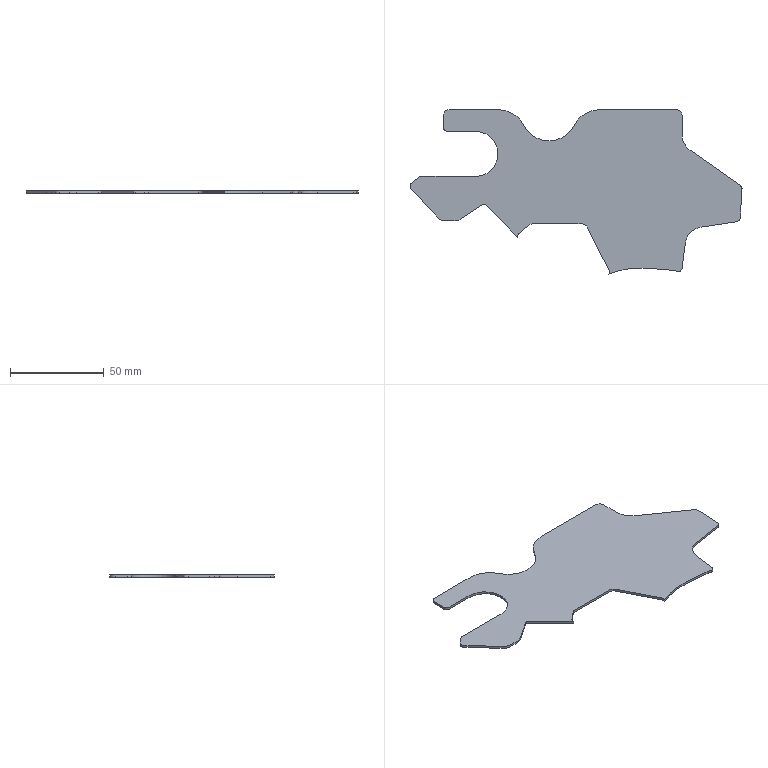Part | STEP file | gslz 2016.10.28-13_id246_x_t | 1 solid | 47 faces | box 176.605 x 87.506 x 1.25 mm | volume 11147 mm3 | cylinder 24 | plane 23 | commonest cylinder face diameters 4 x9 6 x5 30 x4 20 x2 3 x1 12 x1